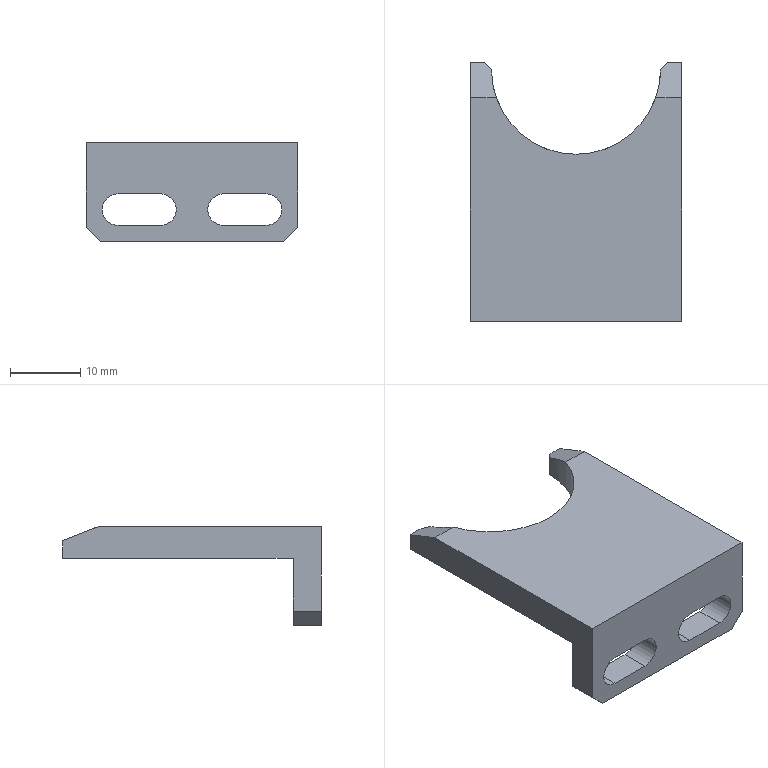Part | STEP file | 0-019 Cover plate locating block (long) | 1 solid | 24 faces | box 30 x 36.7 x 14 mm | volume 4576 mm3 | plane 19 | cylinder 5 | commonest cylinder face diameters 4.5 x4 24 x1